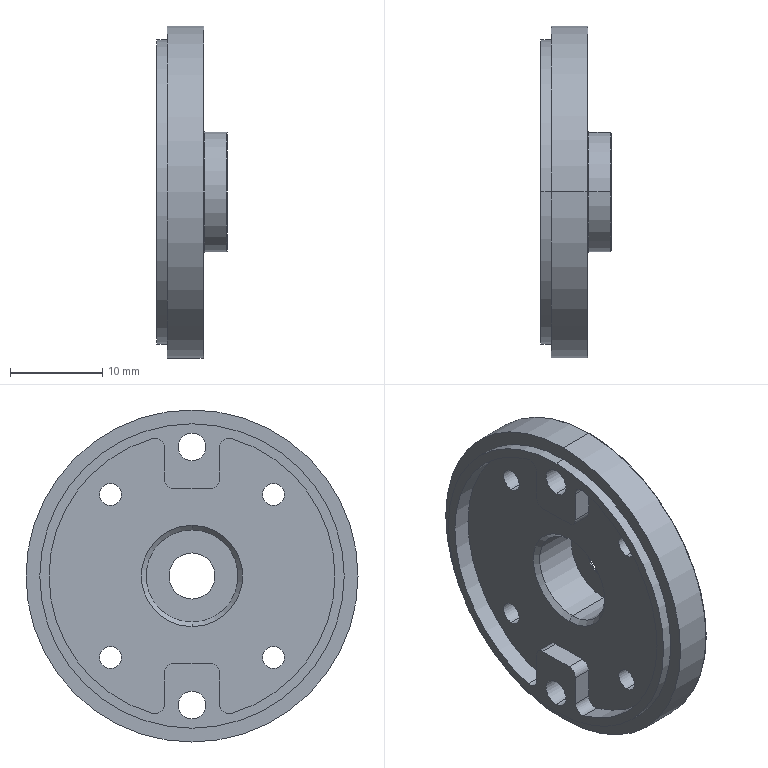Part | SolidWorks | features BaseBody 1 | 1 solid | 62 faces | box 7.6 x 36 x 36 mm | volume 3322 mm3 | cylinder 38 | plane 14 | torus 6 | cone 4 | commonest cylinder face diameters 2 x10 2.4 x8 3 x4 5.5 x4 5 x2 10 x2